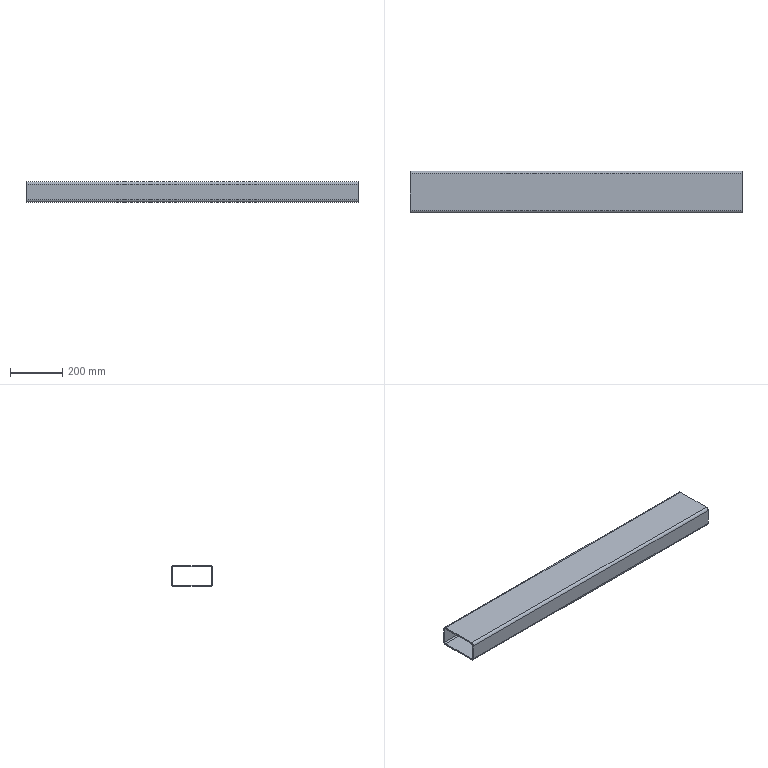Part | SolidWorks | features BaseBody 1 | 1 solid | 18 faces | box 1270 x 160 x 80 mm | volume 2839237 mm3 | plane 10 | cylinder 8 | commonest cylinder face diameters 10 x4 20 x4
STEP:
#1=CARTESIAN_POINT('',(-635.,70.,-40.));
#2=VERTEX_POINT('',#1);
#3=CARTESIAN_POINT('',(-635.,80.,-30.));
#4=VERTEX_POINT('',#3);
#5=CARTESIAN_POINT('',(-635.,70.,-30.));
#6=DIRECTION('',(1.,0.,0.));
#7=DIRECTION('',(0.,0.,-1.));
#8=AXIS2_PLACEMENT_3D('',#5,#6,#7);
#9=CIRCLE('',#8,10.);
#10=EDGE_CURVE('',#2,#4,#9,.T.);
#11=ORIENTED_EDGE('',*,*,#10,.T.);
#12=CARTESIAN_POINT('',(635.,80.,-30.));
#13=VERTEX_POINT('',#12);
#14=CARTESIAN_POINT('',(635.,80.,-30.));
#15=DIRECTION('',(-1.,0.,0.));
#16=VECTOR('',#15,1000.);
#17=LINE('',#14,#16);
#18=EDGE_CURVE('',#13,#4,#17,.T.);
#19=ORIENTED_EDGE('',*,*,#18,.F.);
#20=CARTESIAN_POINT('',(635.,70.,-40.));
#21=VERTEX_POINT('',#20);
#22=CARTESIAN_POINT('',(635.,70.,-30.));
#23=DIRECTION('',(1.,0.,0.));
#24=DIRECTION('',(0.,0.,-1.));
#25=AXIS2_PLACEMENT_3D('',#22,#23,#24);
#26=CIRCLE('',#25,10.);
#27=EDGE_CURVE('',#21,#13,#26,.T.);
#28=ORIENTED_EDGE('',*,*,#27,.F.);
#29=CARTESIAN_POINT('',(635.,70.,-40.));
#30=DIRECTION('',(-1.,0.,0.));
#31=VECTOR('',#30,1000.);
#32=LINE('',#29,#31);
#33=EDGE_CURVE('',#21,#2,#32,.T.);
#34=ORIENTED_EDGE('',*,*,#33,.T.);
#35=EDGE_LOOP('',(#11,#19,#28,#34));
#36=FACE_OUTER_BOUND('',#35,.T.);
#37=CARTESIAN_POINT('',(635.,70.,-30.));
#38=DIRECTION('',(-1.,0.,0.));
#39=DIRECTION('',(0.,0.,1.));
#40=AXIS2_PLACEMENT_3D('',#37,#38,#39);
#41=CYLINDRICAL_SURFACE('',#40,10.);
#42=ADVANCED_FACE('',(#36),#41,.T.);
#43=CARTESIAN_POINT('',(-635.,80.,30.));
#44=VERTEX_POINT('',#43);
#45=CARTESIAN_POINT('',(-635.,80.,-30.));
#46=DIRECTION('',(0.,0.,1.));
#47=VECTOR('',#46,1000.);
#48=LINE('',#45,#47);
#49=EDGE_CURVE('',#4,#44,#48,.T.);
#50=ORIENTED_EDGE('',*,*,#49,.T.);
#51=CARTESIAN_POINT('',(635.,80.,30.));
#52=VERTEX_POINT('',#51);
#53=CARTESIAN_POINT('',(635.,80.,30.));
#54=DIRECTION('',(-1.,0.,0.));
#55=VECTOR('',#54,1000.);
#56=LINE('',#53,#55);
#57=EDGE_CURVE('',#52,#44,#56,.T.);
#58=ORIENTED_EDGE('',*,*,#57,.F.);
#59=CARTESIAN_POINT('',(635.,80.,-30.));
#60=DIRECTION('',(0.,0.,1.));
#61=VECTOR('',#60,1000.);
#62=LINE('',#59,#61);
#63=EDGE_CURVE('',#13,#52,#62,.T.);
#64=ORIENTED_EDGE('',*,*,#63,.F.);
#65=ORIENTED_EDGE('',*,*,#18,.T.);
#66=EDGE_LOOP('',(#50,#58,#64,#65));
#67=FACE_OUTER_BOUND('',#66,.T.);
#68=CARTESIAN_POINT('',(635.,80.,-30.));
#69=DIRECTION('',(0.,-1.,0.));
#70=DIRECTION('',(0.,0.,-1.));
#71=AXIS2_PLACEMENT_3D('',#68,#69,#70);
#72=PLANE('',#71);
#73=ADVANCED_FACE('',(#67),#72,.F.);
#74=CARTESIAN_POINT('',(-635.,70.,40.));
#75=VERTEX_POINT('',#74);
#76=CARTESIAN_POINT('',(-635.,70.,30.));
#77=DIRECTION('',(1.,0.,0.));
#78=DIRECTION('',(0.,0.,-1.));
#79=AXIS2_PLACEMENT_3D('',#76,#77,#78);
#80=CIRCLE('',#79,10.);
#81=EDGE_CURVE('',#44,#75,#80,.T.);
#82=ORIENTED_EDGE('',*,*,#81,.T.);
#83=CARTESIAN_POINT('',(635.,70.,40.));
#84=VERTEX_POINT('',#83);
#85=CARTESIAN_POINT('',(635.,70.,40.));
#86=DIRECTION('',(-1.,0.,0.));
#87=VECTOR('',#86,1000.);
#88=LINE('',#85,#87);
#89=EDGE_CURVE('',#84,#75,#88,.T.);
#90=ORIENTED_EDGE('',*,*,#89,.F.);
#91=CARTESIAN_POINT('',(635.,70.,30.));
#92=DIRECTION('',(1.,0.,0.));
#93=DIRECTION('',(0.,0.,-1.));
#94=AXIS2_PLACEMENT_3D('',#91,#92,#93);
#95=CIRCLE('',#94,10.);
#96=EDGE_CURVE('',#52,#84,#95,.T.);
#97=ORIENTED_EDGE('',*,*,#96,.F.);
#98=ORIENTED_EDGE('',*,*,#57,.T.);
#99=EDGE_LOOP('',(#82,#90,#97,#98));
#100=FACE_OUTER_BOUND('',#99,.T.);
#101=CARTESIAN_POINT('',(635.,70.,30.));
#102=DIRECTION('',(-1.,0.,0.));
#103=DIRECTION('',(0.,0.,1.));
#104=AXIS2_PLACEMENT_3D('',#101,#102,#103);
#105=CYLINDRICAL_SURFACE('',#104,10.);
#106=ADVANCED_FACE('',(#100),#105,.T.);
#107=CARTESIAN_POINT('',(-635.,-70.,40.));
#108=VERTEX_POINT('',#107);
#109=CARTESIAN_POINT('',(-635.,-70.,40.));
#110=DIRECTION('',(0.,-1.,0.));
#111=VECTOR('',#110,1000.);
#112=LINE('',#109,#111);
#113=EDGE_CURVE('',#75,#108,#112,.T.);
#114=ORIENTED_EDGE('',*,*,#113,.T.);
#115=CARTESIAN_POINT('',(635.,-70.,40.));
#116=VERTEX_POINT('',#115);
#117=CARTESIAN_POINT('',(635.,-70.,40.));
#118=DIRECTION('',(-1.,0.,0.));
#119=VECTOR('',#118,1000.);
#120=LINE('',#117,#119);
#121=EDGE_CURVE('',#116,#108,#120,.T.);
#122=ORIENTED_EDGE('',*,*,#121,.F.);
#123=CARTESIAN_POINT('',(635.,-70.,40.));
#124=DIRECTION('',(0.,-1.,0.));
#125=VECTOR('',#124,1000.);
#126=LINE('',#123,#125);
#127=EDGE_CURVE('',#84,#116,#126,.T.);
#128=ORIENTED_EDGE('',*,*,#127,.F.);
#129=ORIENTED_EDGE('',*,*,#89,.T.);
#130=EDGE_LOOP('',(#114,#122,#128,#129));
#131=FACE_OUTER_BOUND('',#130,.T.);
#132=CARTESIAN_POINT('',(635.,-70.,40.));
#133=DIRECTION('',(0.,0.,-1.));
#134=DIRECTION('',(0.,1.,0.));
#135=AXIS2_PLACEMENT_3D('',#132,#133,#134);
#136=PLANE('',#135);
#137=ADVANCED_FACE('',(#131),#136,.F.);
#138=CARTESIAN_POINT('',(-635.,-80.,30.));
#139=VERTEX_POINT('',#138);
#140=CARTESIAN_POINT('',(-635.,-70.,30.));
#141=DIRECTION('',(1.,0.,0.));
#142=DIRECTION('',(0.,0.,-1.));
#143=AXIS2_PLACEMENT_3D('',#140,#141,#142);
#144=CIRCLE('',#143,10.);
#145=EDGE_CURVE('',#108,#139,#144,.T.);
#146=ORIENTED_EDGE('',*,*,#145,.T.);
#147=CARTESIAN_POINT('',(635.,-80.,30.));
#148=VERTEX_POINT('',#147);
#149=CARTESIAN_POINT('',(635.,-80.,30.));
#150=DIRECTION('',(-1.,0.,0.));
#151=VECTOR('',#150,1000.);
#152=LINE('',#149,#151);
#153=EDGE_CURVE('',#148,#139,#152,.T.);
#154=ORIENTED_EDGE('',*,*,#153,.F.);
#155=CARTESIAN_POINT('',(635.,-70.,30.));
#156=DIRECTION('',(1.,0.,0.));
#157=DIRECTION('',(0.,0.,-1.));
#158=AXIS2_PLACEMENT_3D('',#155,#156,#157);
#159=CIRCLE('',#158,10.);
#160=EDGE_CURVE('',#116,#148,#159,.T.);
#161=ORIENTED_EDGE('',*,*,#160,.F.);
#162=ORIENTED_EDGE('',*,*,#121,.T.);
#163=EDGE_LOOP('',(#146,#154,#161,#162));
#164=FACE_OUTER_BOUND('',#163,.T.);
#165=CARTESIAN_POINT('',(635.,-70.,30.));
#166=DIRECTION('',(-1.,0.,0.));
#167=DIRECTION('',(0.,0.,1.));
#168=AXIS2_PLACEMENT_3D('',#165,#166,#167);
#169=CYLINDRICAL_SURFACE('',#168,10.);
#170=ADVANCED_FACE('',(#164),#169,.T.);
#171=CARTESIAN_POINT('',(-635.,-80.,-30.));
#172=VERTEX_POINT('',#171);
#173=CARTESIAN_POINT('',(-635.,-80.,30.));
#174=DIRECTION('',(0.,0.,-1.));
#175=VECTOR('',#174,1000.);
#176=LINE('',#173,#175);
#177=EDGE_CURVE('',#139,#172,#176,.T.);
#178=ORIENTED_EDGE('',*,*,#177,.T.);
#179=CARTESIAN_POINT('',(635.,-80.,-30.));
#180=VERTEX_POINT('',#179);
#181=CARTESIAN_POINT('',(635.,-80.,-30.));
#182=DIRECTION('',(-1.,0.,0.));
#183=VECTOR('',#182,1000.);
#184=LINE('',#181,#183);
#185=EDGE_CURVE('',#180,#172,#184,.T.);
#186=ORIENTED_EDGE('',*,*,#185,.F.);
#187=CARTESIAN_POINT('',(635.,-80.,30.));
#188=DIRECTION('',(0.,0.,-1.));
#189=VECTOR('',#188,1000.);
#190=LINE('',#187,#189);
#191=EDGE_CURVE('',#148,#180,#190,.T.);
#192=ORIENTED_EDGE('',*,*,#191,.F.);
#193=ORIENTED_EDGE('',*,*,#153,.T.);
#194=EDGE_LOOP('',(#178,#186,#192,#193));
#195=FACE_OUTER_BOUND('',#194,.T.);
#196=CARTESIAN_POINT('',(635.,-80.,30.));
#197=DIRECTION('',(0.,1.,0.));
#198=DIRECTION('',(0.,0.,1.));
#199=AXIS2_PLACEMENT_3D('',#196,#197,#198);
#200=PLANE('',#199);
#201=ADVANCED_FACE('',(#195),#200,.F.);
#202=CARTESIAN_POINT('',(-635.,-70.,-40.));
#203=VERTEX_POINT('',#202);
#204=CARTESIAN_POINT('',(-635.,-70.,-30.));
#205=DIRECTION('',(1.,0.,0.));
#206=DIRECTION('',(0.,0.,-1.));
#207=AXIS2_PLACEMENT_3D('',#204,#205,#206);
#208=CIRCLE('',#207,10.);
#209=EDGE_CURVE('',#172,#203,#208,.T.);
#210=ORIENTED_EDGE('',*,*,#209,.T.);
#211=CARTESIAN_POINT('',(635.,-70.,-40.));
#212=VERTEX_POINT('',#211);
#213=CARTESIAN_POINT('',(635.,-70.,-40.));
#214=DIRECTION('',(-1.,0.,0.));
#215=VECTOR('',#214,1000.);
#216=LINE('',#213,#215);
#217=EDGE_CURVE('',#212,#203,#216,.T.);
#218=ORIENTED_EDGE('',*,*,#217,.F.);
#219=CARTESIAN_POINT('',(635.,-70.,-30.));
#220=DIRECTION('',(1.,0.,0.));
#221=DIRECTION('',(0.,0.,-1.));
#222=AXIS2_PLACEMENT_3D('',#219,#220,#221);
#223=CIRCLE('',#222,10.);
#224=EDGE_CURVE('',#180,#212,#223,.T.);
#225=ORIENTED_EDGE('',*,*,#224,.F.);
#226=ORIENTED_EDGE('',*,*,#185,.T.);
#227=EDGE_LOOP('',(#210,#218,#225,#226));
#228=FACE_OUTER_BOUND('',#227,.T.);
#229=CARTESIAN_POINT('',(635.,-70.,-30.));
#230=DIRECTION('',(-1.,0.,0.));
#231=DIRECTION('',(0.,0.,1.));
#232=AXIS2_PLACEMENT_3D('',#229,#230,#231);
#233=CYLINDRICAL_SURFACE('',#232,10.);
#234=ADVANCED_FACE('',(#228),#233,.T.);
#235=CARTESIAN_POINT('',(-635.,75.,30.));
#236=VERTEX_POINT('',#235);
#237=CARTESIAN_POINT('',(-635.,70.,35.));
#238=VERTEX_POINT('',#237);
#239=CARTESIAN_POINT('',(-635.,70.,30.));
#240=DIRECTION('',(1.,0.,0.));
#241=DIRECTION('',(0.,0.,-1.));
#242=AXIS2_PLACEMENT_3D('',#239,#240,#241);
#243=CIRCLE('',#242,5.);
#244=EDGE_CURVE('',#236,#238,#243,.T.);
#245=ORIENTED_EDGE('',*,*,#244,.F.);
#246=CARTESIAN_POINT('',(635.,75.,30.));
#247=VERTEX_POINT('',#246);
#248=CARTESIAN_POINT('',(635.,75.,30.));
#249=DIRECTION('',(-1.,0.,0.));
#250=VECTOR('',#249,1000.);
#251=LINE('',#248,#250);
#252=EDGE_CURVE('',#247,#236,#251,.T.);
#253=ORIENTED_EDGE('',*,*,#252,.F.);
#254=CARTESIAN_POINT('',(635.,70.,35.));
#255=VERTEX_POINT('',#254);
#256=CARTESIAN_POINT('',(635.,70.,30.));
#257=DIRECTION('',(1.,0.,0.));
#258=DIRECTION('',(0.,0.,-1.));
#259=AXIS2_PLACEMENT_3D('',#256,#257,#258);
#260=CIRCLE('',#259,5.);
#261=EDGE_CURVE('',#247,#255,#260,.T.);
#262=ORIENTED_EDGE('',*,*,#261,.T.);
#263=CARTESIAN_POINT('',(635.,70.,35.));
#264=DIRECTION('',(-1.,0.,0.));
#265=VECTOR('',#264,1000.);
#266=LINE('',#263,#265);
#267=EDGE_CURVE('',#255,#238,#266,.T.);
#268=ORIENTED_EDGE('',*,*,#267,.T.);
#269=EDGE_LOOP('',(#245,#253,#262,#268));
#270=FACE_OUTER_BOUND('',#269,.T.);
#271=CARTESIAN_POINT('',(635.,70.,30.));
#272=DIRECTION('',(-1.,0.,0.));
#273=DIRECTION('',(0.,0.,1.));
#274=AXIS2_PLACEMENT_3D('',#271,#272,#273);
#275=CYLINDRICAL_SURFACE('',#274,5.);
#276=ADVANCED_FACE('',(#270),#275,.F.);
#277=CARTESIAN_POINT('',(-635.,75.,-30.));
#278=VERTEX_POINT('',#277);
#279=CARTESIAN_POINT('',(-635.,75.,-30.));
#280=DIRECTION('',(0.,0.,1.));
#281=VECTOR('',#280,1000.);
#282=LINE('',#279,#281);
#283=EDGE_CURVE('',#278,#236,#282,.T.);
#284=ORIENTED_EDGE('',*,*,#283,.F.);
#285=CARTESIAN_POINT('',(635.,75.,-30.));
#286=VERTEX_POINT('',#285);
#287=CARTESIAN_POINT('',(635.,75.,-30.));
#288=DIRECTION('',(-1.,0.,0.));
#289=VECTOR('',#288,1000.);
#290=LINE('',#287,#289);
#291=EDGE_CURVE('',#286,#278,#290,.T.);
#292=ORIENTED_EDGE('',*,*,#291,.F.);
#293=CARTESIAN_POINT('',(635.,75.,-30.));
#294=DIRECTION('',(0.,0.,1.));
#295=VECTOR('',#294,1000.);
#296=LINE('',#293,#295);
#297=EDGE_CURVE('',#286,#247,#296,.T.);
#298=ORIENTED_EDGE('',*,*,#297,.T.);
#299=ORIENTED_EDGE('',*,*,#252,.T.);
#300=EDGE_LOOP('',(#284,#292,#298,#299));
#301=FACE_OUTER_BOUND('',#300,.T.);
#302=CARTESIAN_POINT('',(635.,75.,-30.));
#303=DIRECTION('',(0.,-1.,0.));
#304=DIRECTION('',(0.,0.,-1.));
#305=AXIS2_PLACEMENT_3D('',#302,#303,#304);
#306=PLANE('',#305);
#307=ADVANCED_FACE('',(#301),#306,.T.);
#308=CARTESIAN_POINT('',(-635.,70.,-35.));
#309=VERTEX_POINT('',#308);
#310=CARTESIAN_POINT('',(-635.,70.,-30.));
#311=DIRECTION('',(1.,0.,0.));
#312=DIRECTION('',(0.,0.,-1.));
#313=AXIS2_PLACEMENT_3D('',#310,#311,#312);
#314=CIRCLE('',#313,5.);
#315=EDGE_CURVE('',#309,#278,#314,.T.);
#316=ORIENTED_EDGE('',*,*,#315,.F.);
#317=CARTESIAN_POINT('',(635.,70.,-35.));
#318=VERTEX_POINT('',#317);
#319=CARTESIAN_POINT('',(635.,70.,-35.));
#320=DIRECTION('',(-1.,0.,0.));
#321=VECTOR('',#320,1000.);
#322=LINE('',#319,#321);
#323=EDGE_CURVE('',#318,#309,#322,.T.);
#324=ORIENTED_EDGE('',*,*,#323,.F.);
#325=CARTESIAN_POINT('',(635.,70.,-30.));
#326=DIRECTION('',(1.,0.,0.));
#327=DIRECTION('',(0.,0.,-1.));
#328=AXIS2_PLACEMENT_3D('',#325,#326,#327);
#329=CIRCLE('',#328,5.);
#330=EDGE_CURVE('',#318,#286,#329,.T.);
#331=ORIENTED_EDGE('',*,*,#330,.T.);
#332=ORIENTED_EDGE('',*,*,#291,.T.);
#333=EDGE_LOOP('',(#316,#324,#331,#332));
#334=FACE_OUTER_BOUND('',#333,.T.);
#335=CARTESIAN_POINT('',(635.,70.,-30.));
#336=DIRECTION('',(-1.,0.,0.));
#337=DIRECTION('',(0.,0.,1.));
#338=AXIS2_PLACEMENT_3D('',#335,#336,#337);
#339=CYLINDRICAL_SURFACE('',#338,5.);
#340=ADVANCED_FACE('',(#334),#339,.F.);
#341=CARTESIAN_POINT('',(-635.,-70.,-35.));
#342=VERTEX_POINT('',#341);
#343=CARTESIAN_POINT('',(-635.,70.,-35.));
#344=DIRECTION('',(0.,1.,0.));
#345=VECTOR('',#344,1000.);
#346=LINE('',#343,#345);
#347=EDGE_CURVE('',#342,#309,#346,.T.);
#348=ORIENTED_EDGE('',*,*,#347,.F.);
#349=CARTESIAN_POINT('',(635.,-70.,-35.));
#350=VERTEX_POINT('',#349);
#351=CARTESIAN_POINT('',(635.,-70.,-35.));
#352=DIRECTION('',(-1.,0.,0.));
#353=VECTOR('',#352,1000.);
#354=LINE('',#351,#353);
#355=EDGE_CURVE('',#350,#342,#354,.T.);
#356=ORIENTED_EDGE('',*,*,#355,.F.);
#357=CARTESIAN_POINT('',(635.,70.,-35.));
#358=DIRECTION('',(0.,1.,0.));
#359=VECTOR('',#358,1000.);
#360=LINE('',#357,#359);
#361=EDGE_CURVE('',#350,#318,#360,.T.);
#362=ORIENTED_EDGE('',*,*,#361,.T.);
#363=ORIENTED_EDGE('',*,*,#323,.T.);
#364=EDGE_LOOP('',(#348,#356,#362,#363));
#365=FACE_OUTER_BOUND('',#364,.T.);
#366=CARTESIAN_POINT('',(635.,70.,-35.));
#367=DIRECTION('',(0.,0.,1.));
#368=DIRECTION('',(1.,0.,0.));
#369=AXIS2_PLACEMENT_3D('',#366,#367,#368);
#370=PLANE('',#369);
#371=ADVANCED_FACE('',(#365),#370,.T.);
#372=CARTESIAN_POINT('',(-635.,-75.,-30.));
#373=VERTEX_POINT('',#372);
#374=CARTESIAN_POINT('',(-635.,-70.,-30.));
#375=DIRECTION('',(1.,0.,0.));
#376=DIRECTION('',(0.,0.,-1.));
#377=AXIS2_PLACEMENT_3D('',#374,#375,#376);
#378=CIRCLE('',#377,5.);
#379=EDGE_CURVE('',#373,#342,#378,.T.);
#380=ORIENTED_EDGE('',*,*,#379,.F.);
#381=CARTESIAN_POINT('',(635.,-75.,-30.));
#382=VERTEX_POINT('',#381);
#383=CARTESIAN_POINT('',(635.,-75.,-30.));
#384=DIRECTION('',(-1.,0.,0.));
#385=VECTOR('',#384,1000.);
#386=LINE('',#383,#385);
#387=EDGE_CURVE('',#382,#373,#386,.T.);
#388=ORIENTED_EDGE('',*,*,#387,.F.);
#389=CARTESIAN_POINT('',(635.,-70.,-30.));
#390=DIRECTION('',(1.,0.,0.));
#391=DIRECTION('',(0.,0.,-1.));
#392=AXIS2_PLACEMENT_3D('',#389,#390,#391);
#393=CIRCLE('',#392,5.);
#394=EDGE_CURVE('',#382,#350,#393,.T.);
#395=ORIENTED_EDGE('',*,*,#394,.T.);
#396=ORIENTED_EDGE('',*,*,#355,.T.);
#397=EDGE_LOOP('',(#380,#388,#395,#396));
#398=FACE_OUTER_BOUND('',#397,.T.);
#399=CARTESIAN_POINT('',(635.,-70.,-30.));
#400=DIRECTION('',(-1.,0.,0.));
#401=DIRECTION('',(0.,0.,1.));
#402=AXIS2_PLACEMENT_3D('',#399,#400,#401);
#403=CYLINDRICAL_SURFACE('',#402,5.);
#404=ADVANCED_FACE('',(#398),#403,.F.);
#405=CARTESIAN_POINT('',(-635.,-75.,30.));
#406=VERTEX_POINT('',#405);
#407=CARTESIAN_POINT('',(-635.,-75.,30.));
#408=DIRECTION('',(0.,0.,-1.));
#409=VECTOR('',#408,1000.);
#410=LINE('',#407,#409);
#411=EDGE_CURVE('',#406,#373,#410,.T.);
#412=ORIENTED_EDGE('',*,*,#411,.F.);
#413=CARTESIAN_POINT('',(635.,-75.,30.));
#414=VERTEX_POINT('',#413);
#415=CARTESIAN_POINT('',(635.,-75.,30.));
#416=DIRECTION('',(-1.,0.,0.));
#417=VECTOR('',#416,1000.);
#418=LINE('',#415,#417);
#419=EDGE_CURVE('',#414,#406,#418,.T.);
#420=ORIENTED_EDGE('',*,*,#419,.F.);
#421=CARTESIAN_POINT('',(635.,-75.,30.));
#422=DIRECTION('',(0.,0.,-1.));
#423=VECTOR('',#422,1000.);
#424=LINE('',#421,#423);
#425=EDGE_CURVE('',#414,#382,#424,.T.);
#426=ORIENTED_EDGE('',*,*,#425,.T.);
#427=ORIENTED_EDGE('',*,*,#387,.T.);
#428=EDGE_LOOP('',(#412,#420,#426,#427));
#429=FACE_OUTER_BOUND('',#428,.T.);
#430=CARTESIAN_POINT('',(635.,-75.,30.));
#431=DIRECTION('',(0.,1.,0.));
#432=DIRECTION('',(0.,0.,1.));
#433=AXIS2_PLACEMENT_3D('',#430,#431,#432);
#434=PLANE('',#433);
#435=ADVANCED_FACE('',(#429),#434,.T.);
#436=CARTESIAN_POINT('',(-635.,-70.,35.));
#437=VERTEX_POINT('',#436);
#438=CARTESIAN_POINT('',(-635.,-70.,30.));
#439=DIRECTION('',(1.,0.,0.));
#440=DIRECTION('',(0.,0.,-1.));
#441=AXIS2_PLACEMENT_3D('',#438,#439,#440);
#442=CIRCLE('',#441,5.);
#443=EDGE_CURVE('',#437,#406,#442,.T.);
#444=ORIENTED_EDGE('',*,*,#443,.F.);
#445=CARTESIAN_POINT('',(635.,-70.,35.));
#446=VERTEX_POINT('',#445);
#447=CARTESIAN_POINT('',(635.,-70.,35.));
#448=DIRECTION('',(-1.,0.,0.));
#449=VECTOR('',#448,1000.);
#450=LINE('',#447,#449);
#451=EDGE_CURVE('',#446,#437,#450,.T.);
#452=ORIENTED_EDGE('',*,*,#451,.F.);
#453=CARTESIAN_POINT('',(635.,-70.,30.));
#454=DIRECTION('',(1.,0.,0.));
#455=DIRECTION('',(0.,0.,-1.));
#456=AXIS2_PLACEMENT_3D('',#453,#454,#455);
#457=CIRCLE('',#456,5.);
#458=EDGE_CURVE('',#446,#414,#457,.T.);
#459=ORIENTED_EDGE('',*,*,#458,.T.);
#460=ORIENTED_EDGE('',*,*,#419,.T.);
#461=EDGE_LOOP('',(#444,#452,#459,#460));
#462=FACE_OUTER_BOUND('',#461,.T.);
#463=CARTESIAN_POINT('',(635.,-70.,30.));
#464=DIRECTION('',(-1.,0.,0.));
#465=DIRECTION('',(0.,0.,1.));
#466=AXIS2_PLACEMENT_3D('',#463,#464,#465);
#467=CYLINDRICAL_SURFACE('',#466,5.);
#468=ADVANCED_FACE('',(#462),#467,.F.);
#469=CARTESIAN_POINT('',(-635.,-70.,35.));
#470=DIRECTION('',(0.,-1.,0.));
#471=VECTOR('',#470,1000.);
#472=LINE('',#469,#471);
#473=EDGE_CURVE('',#238,#437,#472,.T.);
#474=ORIENTED_EDGE('',*,*,#473,.F.);
#475=ORIENTED_EDGE('',*,*,#267,.F.);
#476=CARTESIAN_POINT('',(635.,-70.,35.));
#477=DIRECTION('',(0.,-1.,0.));
#478=VECTOR('',#477,1000.);
#479=LINE('',#476,#478);
#480=EDGE_CURVE('',#255,#446,#479,.T.);
#481=ORIENTED_EDGE('',*,*,#480,.T.);
#482=ORIENTED_EDGE('',*,*,#451,.T.);
#483=EDGE_LOOP('',(#474,#475,#481,#482));
#484=FACE_OUTER_BOUND('',#483,.T.);
#485=CARTESIAN_POINT('',(635.,-70.,35.));
#486=DIRECTION('',(0.,0.,-1.));
#487=DIRECTION('',(0.,1.,0.));
#488=AXIS2_PLACEMENT_3D('',#485,#486,#487);
#489=PLANE('',#488);
#490=ADVANCED_FACE('',(#484),#489,.T.);
#491=CARTESIAN_POINT('',(-635.,70.,-40.));
#492=DIRECTION('',(0.,1.,0.));
#493=VECTOR('',#492,1000.);
#494=LINE('',#491,#493);
#495=EDGE_CURVE('',#203,#2,#494,.T.);
#496=ORIENTED_EDGE('',*,*,#495,.T.);
#497=ORIENTED_EDGE('',*,*,#33,.F.);
#498=CARTESIAN_POINT('',(635.,70.,-40.));
#499=DIRECTION('',(0.,1.,0.));
#500=VECTOR('',#499,1000.);
#501=LINE('',#498,#500);
#502=EDGE_CURVE('',#212,#21,#501,.T.);
#503=ORIENTED_EDGE('',*,*,#502,.F.);
#504=ORIENTED_EDGE('',*,*,#217,.T.);
#505=EDGE_LOOP('',(#496,#497,#503,#504));
#506=FACE_OUTER_BOUND('',#505,.T.);
#507=CARTESIAN_POINT('',(635.,70.,-40.));
#508=DIRECTION('',(0.,0.,1.));
#509=DIRECTION('',(1.,0.,0.));
#510=AXIS2_PLACEMENT_3D('',#507,#508,#509);
#511=PLANE('',#510);
#512=ADVANCED_FACE('',(#506),#511,.F.);
#513=ORIENTED_EDGE('',*,*,#261,.F.);
#514=ORIENTED_EDGE('',*,*,#297,.F.);
#515=ORIENTED_EDGE('',*,*,#330,.F.);
#516=ORIENTED_EDGE('',*,*,#361,.F.);
#517=ORIENTED_EDGE('',*,*,#394,.F.);
#518=ORIENTED_EDGE('',*,*,#425,.F.);
#519=ORIENTED_EDGE('',*,*,#458,.F.);
#520=ORIENTED_EDGE('',*,*,#480,.F.);
#521=EDGE_LOOP('',(#513,#514,#515,#516,#517,#518,#519,#520));
#522=FACE_BOUND('',#521,.T.);
#523=ORIENTED_EDGE('',*,*,#27,.T.);
#524=ORIENTED_EDGE('',*,*,#63,.T.);
#525=ORIENTED_EDGE('',*,*,#96,.T.);
#526=ORIENTED_EDGE('',*,*,#127,.T.);
#527=ORIENTED_EDGE('',*,*,#160,.T.);
#528=ORIENTED_EDGE('',*,*,#191,.T.);
#529=ORIENTED_EDGE('',*,*,#224,.T.);
#530=ORIENTED_EDGE('',*,*,#502,.T.);
#531=EDGE_LOOP('',(#523,#524,#525,#526,#527,#528,#529,#530));
#532=FACE_OUTER_BOUND('',#531,.T.);
#533=CARTESIAN_POINT('',(635.,70.,-30.));
#534=DIRECTION('',(1.,0.,0.));
#535=DIRECTION('',(0.,0.,-1.));
#536=AXIS2_PLACEMENT_3D('',#533,#534,#535);
#537=PLANE('',#536);
#538=ADVANCED_FACE('',(#522,#532),#537,.T.);
#539=ORIENTED_EDGE('',*,*,#244,.T.);
#540=ORIENTED_EDGE('',*,*,#473,.T.);
#541=ORIENTED_EDGE('',*,*,#443,.T.);
#542=ORIENTED_EDGE('',*,*,#411,.T.);
#543=ORIENTED_EDGE('',*,*,#379,.T.);
#544=ORIENTED_EDGE('',*,*,#347,.T.);
#545=ORIENTED_EDGE('',*,*,#315,.T.);
#546=ORIENTED_EDGE('',*,*,#283,.T.);
#547=EDGE_LOOP('',(#539,#540,#541,#542,#543,#544,#545,#546));
#548=FACE_BOUND('',#547,.T.);
#549=ORIENTED_EDGE('',*,*,#10,.F.);
#550=ORIENTED_EDGE('',*,*,#495,.F.);
#551=ORIENTED_EDGE('',*,*,#209,.F.);
#552=ORIENTED_EDGE('',*,*,#177,.F.);
#553=ORIENTED_EDGE('',*,*,#145,.F.);
#554=ORIENTED_EDGE('',*,*,#113,.F.);
#555=ORIENTED_EDGE('',*,*,#81,.F.);
#556=ORIENTED_EDGE('',*,*,#49,.F.);
#557=EDGE_LOOP('',(#549,#550,#551,#552,#553,#554,#555,#556));
#558=FACE_OUTER_BOUND('',#557,.T.);
#559=CARTESIAN_POINT('',(-635.,70.,-30.));
#560=DIRECTION('',(1.,0.,0.));
#561=DIRECTION('',(0.,0.,-1.));
#562=AXIS2_PLACEMENT_3D('',#559,#560,#561);
#563=PLANE('',#562);
#564=ADVANCED_FACE('',(#548,#558),#563,.F.);
#565=CLOSED_SHELL('',(#42,#73,#106,#137,#170,#201,#234,#276,#307,#340,#371,#404,#435,#468,#490,#512,#538,#564));
#566=MANIFOLD_SOLID_BREP('',#565);
#567=CARTESIAN_POINT('',(0.,0.,0.));
#568=DIRECTION('',(0.,0.,1.));
#569=DIRECTION('',(1.,0.,0.));
#570=AXIS2_PLACEMENT_3D('',#567,#568,#569);
#571=(LENGTH_UNIT()NAMED_UNIT(*)SI_UNIT(.MILLI.,.METRE.));
#572=UNCERTAINTY_MEASURE_WITH_UNIT(LENGTH_MEASURE(0.00001),#571,'','');
#573=(NAMED_UNIT(*)PLANE_ANGLE_UNIT()SI_UNIT($,.RADIAN.));
#574=(NAMED_UNIT(*)SI_UNIT($,.STERADIAN.)SOLID_ANGLE_UNIT());
#575=(GEOMETRIC_REPRESENTATION_CONTEXT(3)GLOBAL_UNCERTAINTY_ASSIGNED_CONTEXT((#572))GLOBAL_UNIT_ASSIGNED_CONTEXT((#571,#573,#574))REPRESENTATION_CONTEXT('',''));
#576=ADVANCED_BREP_SHAPE_REPRESENTATION('',(#566,#570),#575);